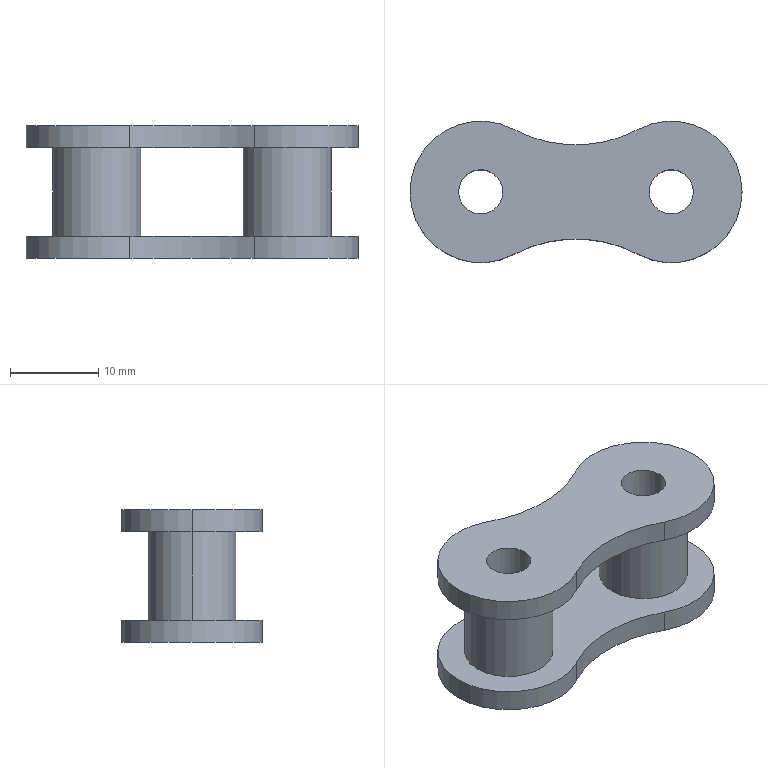Part | SolidWorks | 1 solid | 22 faces | box 37.56 x 16 x 15 mm | volume 3392 mm3 | cylinder 18 | plane 4 | commonest cylinder face diameters 16 x6 5 x4 10 x4 30 x4
STEP:
#1=CARTESIAN_POINT('',(3.75,-7.067,7.5));
#2=VERTEX_POINT('',#1);
#3=CARTESIAN_POINT('',(-8.,0.,7.5));
#4=VERTEX_POINT('',#3);
#5=CARTESIAN_POINT('',(0.,0.,7.5));
#6=DIRECTION('',(0.,0.,-1.));
#7=DIRECTION('',(-1.,0.,0.));
#8=AXIS2_PLACEMENT_3D('',#5,#6,#7);
#9=CIRCLE('',#8,8.);
#10=EDGE_CURVE('',#2,#4,#9,.T.);
#11=ORIENTED_EDGE('',*,*,#10,.T.);
#12=CARTESIAN_POINT('',(-8.,0.,5.));
#13=VERTEX_POINT('',#12);
#14=CARTESIAN_POINT('',(-8.,0.,7.5));
#15=DIRECTION('',(0.,0.,-1.));
#16=VECTOR('',#15,1000.);
#17=LINE('',#14,#16);
#18=EDGE_CURVE('',#4,#13,#17,.T.);
#19=ORIENTED_EDGE('',*,*,#18,.T.);
#20=CARTESIAN_POINT('',(3.75,-7.067,5.));
#21=VERTEX_POINT('',#20);
#22=CARTESIAN_POINT('',(0.,0.,5.));
#23=DIRECTION('',(0.,0.,-1.));
#24=DIRECTION('',(-1.,0.,0.));
#25=AXIS2_PLACEMENT_3D('',#22,#23,#24);
#26=CIRCLE('',#25,8.);
#27=EDGE_CURVE('',#21,#13,#26,.T.);
#28=ORIENTED_EDGE('',*,*,#27,.F.);
#29=CARTESIAN_POINT('',(3.75,-7.067,7.5));
#30=DIRECTION('',(0.,0.,-1.));
#31=VECTOR('',#30,1000.);
#32=LINE('',#29,#31);
#33=EDGE_CURVE('',#2,#21,#32,.T.);
#34=ORIENTED_EDGE('',*,*,#33,.F.);
#35=EDGE_LOOP('',(#11,#19,#28,#34));
#36=FACE_OUTER_BOUND('',#35,.T.);
#37=CARTESIAN_POINT('',(0.,0.,7.5));
#38=DIRECTION('',(0.,0.,-1.));
#39=DIRECTION('',(-1.,0.,0.));
#40=AXIS2_PLACEMENT_3D('',#37,#38,#39);
#41=CYLINDRICAL_SURFACE('',#40,8.);
#42=ADVANCED_FACE('',(#36),#41,.T.);
#43=CARTESIAN_POINT('',(26.56,0.,5.));
#44=VERTEX_POINT('',#43);
#45=CARTESIAN_POINT('',(16.56,0.,5.));
#46=VERTEX_POINT('',#45);
#47=CARTESIAN_POINT('',(21.56,0.,5.));
#48=DIRECTION('',(0.,0.,1.));
#49=DIRECTION('',(1.,0.,0.));
#50=AXIS2_PLACEMENT_3D('',#47,#48,#49);
#51=CIRCLE('',#50,5.);
#52=EDGE_CURVE('',#44,#46,#51,.T.);
#53=ORIENTED_EDGE('',*,*,#52,.F.);
#54=CARTESIAN_POINT('',(26.56,0.,-5.));
#55=VERTEX_POINT('',#54);
#56=CARTESIAN_POINT('',(26.56,0.,5.));
#57=DIRECTION('',(0.,0.,-1.));
#58=VECTOR('',#57,1000.);
#59=LINE('',#56,#58);
#60=EDGE_CURVE('',#44,#55,#59,.T.);
#61=ORIENTED_EDGE('',*,*,#60,.T.);
#62=CARTESIAN_POINT('',(16.56,0.,-5.));
#63=VERTEX_POINT('',#62);
#64=CARTESIAN_POINT('',(21.56,0.,-5.));
#65=DIRECTION('',(0.,0.,1.));
#66=DIRECTION('',(-1.,0.,0.));
#67=AXIS2_PLACEMENT_3D('',#64,#65,#66);
#68=CIRCLE('',#67,5.);
#69=EDGE_CURVE('',#55,#63,#68,.T.);
#70=ORIENTED_EDGE('',*,*,#69,.T.);
#71=CARTESIAN_POINT('',(16.56,0.,5.));
#72=DIRECTION('',(0.,0.,-1.));
#73=VECTOR('',#72,1000.);
#74=LINE('',#71,#73);
#75=EDGE_CURVE('',#46,#63,#74,.T.);
#76=ORIENTED_EDGE('',*,*,#75,.F.);
#77=EDGE_LOOP('',(#53,#61,#70,#76));
#78=FACE_OUTER_BOUND('',#77,.T.);
#79=CARTESIAN_POINT('',(21.56,0.,5.));
#80=DIRECTION('',(0.,0.,-1.));
#81=DIRECTION('',(-1.,0.,0.));
#82=AXIS2_PLACEMENT_3D('',#79,#80,#81);
#83=CYLINDRICAL_SURFACE('',#82,5.);
#84=ADVANCED_FACE('',(#78),#83,.T.);
#85=CARTESIAN_POINT('',(24.06,0.,-7.5));
#86=VERTEX_POINT('',#85);
#87=CARTESIAN_POINT('',(19.06,0.,-7.5));
#88=VERTEX_POINT('',#87);
#89=CARTESIAN_POINT('',(21.56,0.,-7.5));
#90=DIRECTION('',(0.,0.,-1.));
#91=DIRECTION('',(-1.,0.,0.));
#92=AXIS2_PLACEMENT_3D('',#89,#90,#91);
#93=CIRCLE('',#92,2.5);
#94=EDGE_CURVE('',#86,#88,#93,.T.);
#95=ORIENTED_EDGE('',*,*,#94,.T.);
#96=CARTESIAN_POINT('',(19.06,0.,7.5));
#97=VERTEX_POINT('',#96);
#98=CARTESIAN_POINT('',(19.06,0.,-7.5));
#99=DIRECTION('',(0.,0.,1.));
#100=VECTOR('',#99,1000.);
#101=LINE('',#98,#100);
#102=EDGE_CURVE('',#88,#97,#101,.T.);
#103=ORIENTED_EDGE('',*,*,#102,.T.);
#104=CARTESIAN_POINT('',(24.06,0.,7.5));
#105=VERTEX_POINT('',#104);
#106=CARTESIAN_POINT('',(21.56,0.,7.5));
#107=DIRECTION('',(0.,0.,-1.));
#108=DIRECTION('',(-1.,0.,0.));
#109=AXIS2_PLACEMENT_3D('',#106,#107,#108);
#110=CIRCLE('',#109,2.5);
#111=EDGE_CURVE('',#105,#97,#110,.T.);
#112=ORIENTED_EDGE('',*,*,#111,.F.);
#113=CARTESIAN_POINT('',(24.06,0.,-7.5));
#114=DIRECTION('',(0.,0.,1.));
#115=VECTOR('',#114,1000.);
#116=LINE('',#113,#115);
#117=EDGE_CURVE('',#86,#105,#116,.T.);
#118=ORIENTED_EDGE('',*,*,#117,.F.);
#119=EDGE_LOOP('',(#95,#103,#112,#118));
#120=FACE_OUTER_BOUND('',#119,.T.);
#121=CARTESIAN_POINT('',(21.56,0.,-7.5));
#122=DIRECTION('',(0.,0.,1.));
#123=DIRECTION('',(1.,0.,0.));
#124=AXIS2_PLACEMENT_3D('',#121,#122,#123);
#125=CYLINDRICAL_SURFACE('',#124,2.5);
#126=ADVANCED_FACE('',(#120),#125,.F.);
#127=CARTESIAN_POINT('',(29.56,0.,-7.5));
#128=VERTEX_POINT('',#127);
#129=CARTESIAN_POINT('',(17.81,-7.067,-7.5));
#130=VERTEX_POINT('',#129);
#131=CARTESIAN_POINT('',(21.56,0.,-7.5));
#132=DIRECTION('',(0.,0.,-1.));
#133=DIRECTION('',(-1.,0.,0.));
#134=AXIS2_PLACEMENT_3D('',#131,#132,#133);
#135=CIRCLE('',#134,8.);
#136=EDGE_CURVE('',#128,#130,#135,.T.);
#137=ORIENTED_EDGE('',*,*,#136,.F.);
#138=CARTESIAN_POINT('',(29.56,0.,-5.));
#139=VERTEX_POINT('',#138);
#140=CARTESIAN_POINT('',(29.56,0.,-7.5));
#141=DIRECTION('',(0.,0.,1.));
#142=VECTOR('',#141,1000.);
#143=LINE('',#140,#142);
#144=EDGE_CURVE('',#128,#139,#143,.T.);
#145=ORIENTED_EDGE('',*,*,#144,.T.);
#146=CARTESIAN_POINT('',(17.81,-7.067,-5.));
#147=VERTEX_POINT('',#146);
#148=CARTESIAN_POINT('',(21.56,0.,-5.));
#149=DIRECTION('',(0.,0.,-1.));
#150=DIRECTION('',(-1.,0.,0.));
#151=AXIS2_PLACEMENT_3D('',#148,#149,#150);
#152=CIRCLE('',#151,8.);
#153=EDGE_CURVE('',#139,#147,#152,.T.);
#154=ORIENTED_EDGE('',*,*,#153,.T.);
#155=CARTESIAN_POINT('',(17.81,-7.067,-7.5));
#156=DIRECTION('',(0.,0.,1.));
#157=VECTOR('',#156,1000.);
#158=LINE('',#155,#157);
#159=EDGE_CURVE('',#130,#147,#158,.T.);
#160=ORIENTED_EDGE('',*,*,#159,.F.);
#161=EDGE_LOOP('',(#137,#145,#154,#160));
#162=FACE_OUTER_BOUND('',#161,.T.);
#163=CARTESIAN_POINT('',(21.56,0.,-7.5));
#164=DIRECTION('',(0.,0.,1.));
#165=DIRECTION('',(1.,0.,0.));
#166=AXIS2_PLACEMENT_3D('',#163,#164,#165);
#167=CYLINDRICAL_SURFACE('',#166,8.);
#168=ADVANCED_FACE('',(#162),#167,.T.);
#169=CARTESIAN_POINT('',(2.5,0.,7.5));
#170=VERTEX_POINT('',#169);
#171=CARTESIAN_POINT('',(-2.5,0.,7.5));
#172=VERTEX_POINT('',#171);
#173=CARTESIAN_POINT('',(0.,0.,7.5));
#174=DIRECTION('',(0.,0.,-1.));
#175=DIRECTION('',(-1.,0.,0.));
#176=AXIS2_PLACEMENT_3D('',#173,#174,#175);
#177=CIRCLE('',#176,2.5);
#178=EDGE_CURVE('',#170,#172,#177,.T.);
#179=ORIENTED_EDGE('',*,*,#178,.F.);
#180=CARTESIAN_POINT('',(2.5,0.,-7.5));
#181=VERTEX_POINT('',#180);
#182=CARTESIAN_POINT('',(2.5,0.,5.));
#183=DIRECTION('',(0.,0.,-1.));
#184=VECTOR('',#183,1000.);
#185=LINE('',#182,#184);
#186=EDGE_CURVE('',#170,#181,#185,.T.);
#187=ORIENTED_EDGE('',*,*,#186,.T.);
#188=CARTESIAN_POINT('',(-2.5,0.,-7.5));
#189=VERTEX_POINT('',#188);
#190=CARTESIAN_POINT('',(0.,0.,-7.5));
#191=DIRECTION('',(0.,0.,-1.));
#192=DIRECTION('',(-1.,0.,0.));
#193=AXIS2_PLACEMENT_3D('',#190,#191,#192);
#194=CIRCLE('',#193,2.5);
#195=EDGE_CURVE('',#181,#189,#194,.T.);
#196=ORIENTED_EDGE('',*,*,#195,.T.);
#197=CARTESIAN_POINT('',(-2.5,0.,5.));
#198=DIRECTION('',(0.,0.,-1.));
#199=VECTOR('',#198,1000.);
#200=LINE('',#197,#199);
#201=EDGE_CURVE('',#172,#189,#200,.T.);
#202=ORIENTED_EDGE('',*,*,#201,.F.);
#203=EDGE_LOOP('',(#179,#187,#196,#202));
#204=FACE_OUTER_BOUND('',#203,.T.);
#205=CARTESIAN_POINT('',(0.,0.,5.));
#206=DIRECTION('',(0.,0.,-1.));
#207=DIRECTION('',(-1.,0.,0.));
#208=AXIS2_PLACEMENT_3D('',#205,#206,#207);
#209=CYLINDRICAL_SURFACE('',#208,2.5);
#210=ADVANCED_FACE('',(#204),#209,.F.);
#211=CARTESIAN_POINT('',(5.,0.,5.));
#212=VERTEX_POINT('',#211);
#213=CARTESIAN_POINT('',(-5.,0.,5.));
#214=VERTEX_POINT('',#213);
#215=CARTESIAN_POINT('',(0.,0.,5.));
#216=DIRECTION('',(0.,0.,1.));
#217=DIRECTION('',(1.,0.,0.));
#218=AXIS2_PLACEMENT_3D('',#215,#216,#217);
#219=CIRCLE('',#218,5.);
#220=EDGE_CURVE('',#212,#214,#219,.T.);
#221=ORIENTED_EDGE('',*,*,#220,.F.);
#222=CARTESIAN_POINT('',(5.,0.,-5.));
#223=VERTEX_POINT('',#222);
#224=CARTESIAN_POINT('',(5.,0.,5.));
#225=DIRECTION('',(0.,0.,-1.));
#226=VECTOR('',#225,1000.);
#227=LINE('',#224,#226);
#228=EDGE_CURVE('',#212,#223,#227,.T.);
#229=ORIENTED_EDGE('',*,*,#228,.T.);
#230=CARTESIAN_POINT('',(-5.,0.,-5.));
#231=VERTEX_POINT('',#230);
#232=CARTESIAN_POINT('',(0.,0.,-5.));
#233=DIRECTION('',(0.,0.,1.));
#234=DIRECTION('',(1.,0.,0.));
#235=AXIS2_PLACEMENT_3D('',#232,#233,#234);
#236=CIRCLE('',#235,5.);
#237=EDGE_CURVE('',#223,#231,#236,.T.);
#238=ORIENTED_EDGE('',*,*,#237,.T.);
#239=CARTESIAN_POINT('',(-5.,0.,5.));
#240=DIRECTION('',(0.,0.,-1.));
#241=VECTOR('',#240,1000.);
#242=LINE('',#239,#241);
#243=EDGE_CURVE('',#214,#231,#242,.T.);
#244=ORIENTED_EDGE('',*,*,#243,.F.);
#245=EDGE_LOOP('',(#221,#229,#238,#244));
#246=FACE_OUTER_BOUND('',#245,.T.);
#247=CARTESIAN_POINT('',(0.,0.,5.));
#248=DIRECTION('',(0.,0.,-1.));
#249=DIRECTION('',(-1.,0.,0.));
#250=AXIS2_PLACEMENT_3D('',#247,#248,#249);
#251=CYLINDRICAL_SURFACE('',#250,5.);
#252=ADVANCED_FACE('',(#246),#251,.T.);
#253=CARTESIAN_POINT('',(3.75,7.067,-5.));
#254=VERTEX_POINT('',#253);
#255=CARTESIAN_POINT('',(17.81,7.067,-5.));
#256=VERTEX_POINT('',#255);
#257=CARTESIAN_POINT('',(10.78,20.317,-5.));
#258=DIRECTION('',(0.,0.,1.));
#259=DIRECTION('',(-1.,0.,0.));
#260=AXIS2_PLACEMENT_3D('',#257,#258,#259);
#261=CIRCLE('',#260,15.);
#262=EDGE_CURVE('',#254,#256,#261,.T.);
#263=ORIENTED_EDGE('',*,*,#262,.F.);
#264=CARTESIAN_POINT('',(3.75,-7.067,-5.));
#265=VERTEX_POINT('',#264);
#266=CARTESIAN_POINT('',(0.,0.,-5.));
#267=DIRECTION('',(0.,0.,-1.));
#268=DIRECTION('',(-1.,0.,0.));
#269=AXIS2_PLACEMENT_3D('',#266,#267,#268);
#270=CIRCLE('',#269,8.);
#271=EDGE_CURVE('',#265,#254,#270,.T.);
#272=ORIENTED_EDGE('',*,*,#271,.F.);
#273=CARTESIAN_POINT('',(10.78,-20.317,-5.));
#274=DIRECTION('',(0.,0.,1.));
#275=DIRECTION('',(1.,0.,0.));
#276=AXIS2_PLACEMENT_3D('',#273,#274,#275);
#277=CIRCLE('',#276,15.);
#278=EDGE_CURVE('',#147,#265,#277,.T.);
#279=ORIENTED_EDGE('',*,*,#278,.F.);
#280=ORIENTED_EDGE('',*,*,#153,.F.);
#281=CARTESIAN_POINT('',(21.56,0.,-5.));
#282=DIRECTION('',(0.,0.,-1.));
#283=DIRECTION('',(-1.,0.,0.));
#284=AXIS2_PLACEMENT_3D('',#281,#282,#283);
#285=CIRCLE('',#284,8.);
#286=EDGE_CURVE('',#256,#139,#285,.T.);
#287=ORIENTED_EDGE('',*,*,#286,.F.);
#288=EDGE_LOOP('',(#263,#272,#279,#280,#287));
#289=FACE_OUTER_BOUND('',#288,.T.);
#290=CARTESIAN_POINT('',(0.,0.,-5.));
#291=DIRECTION('',(0.,0.,1.));
#292=DIRECTION('',(1.,0.,0.));
#293=AXIS2_PLACEMENT_3D('',#290,#291,#292);
#294=CIRCLE('',#293,5.);
#295=EDGE_CURVE('',#231,#223,#294,.T.);
#296=ORIENTED_EDGE('',*,*,#295,.F.);
#297=ORIENTED_EDGE('',*,*,#237,.F.);
#298=EDGE_LOOP('',(#296,#297));
#299=FACE_BOUND('',#298,.T.);
#300=CARTESIAN_POINT('',(21.56,0.,-5.));
#301=DIRECTION('',(0.,0.,1.));
#302=DIRECTION('',(-1.,0.,0.));
#303=AXIS2_PLACEMENT_3D('',#300,#301,#302);
#304=CIRCLE('',#303,5.);
#305=EDGE_CURVE('',#63,#55,#304,.T.);
#306=ORIENTED_EDGE('',*,*,#305,.F.);
#307=ORIENTED_EDGE('',*,*,#69,.F.);
#308=EDGE_LOOP('',(#306,#307));
#309=FACE_BOUND('',#308,.T.);
#310=CARTESIAN_POINT('',(5.39,10.159,-5.));
#311=DIRECTION('',(0.,0.,-1.));
#312=DIRECTION('',(-1.,0.,0.));
#313=AXIS2_PLACEMENT_3D('',#310,#311,#312);
#314=PLANE('',#313);
#315=ADVANCED_FACE('',(#289,#299,#309),#314,.F.);
#316=ORIENTED_EDGE('',*,*,#228,.F.);
#317=CARTESIAN_POINT('',(0.,0.,5.));
#318=DIRECTION('',(0.,0.,1.));
#319=DIRECTION('',(1.,0.,0.));
#320=AXIS2_PLACEMENT_3D('',#317,#318,#319);
#321=CIRCLE('',#320,5.);
#322=EDGE_CURVE('',#214,#212,#321,.T.);
#323=ORIENTED_EDGE('',*,*,#322,.F.);
#324=ORIENTED_EDGE('',*,*,#243,.T.);
#325=ORIENTED_EDGE('',*,*,#295,.T.);
#326=EDGE_LOOP('',(#316,#323,#324,#325));
#327=FACE_OUTER_BOUND('',#326,.T.);
#328=CARTESIAN_POINT('',(0.,0.,5.));
#329=DIRECTION('',(0.,0.,-1.));
#330=DIRECTION('',(-1.,0.,0.));
#331=AXIS2_PLACEMENT_3D('',#328,#329,#330);
#332=CYLINDRICAL_SURFACE('',#331,5.);
#333=ADVANCED_FACE('',(#327),#332,.T.);
#334=ORIENTED_EDGE('',*,*,#186,.F.);
#335=CARTESIAN_POINT('',(0.,0.,7.5));
#336=DIRECTION('',(0.,0.,-1.));
#337=DIRECTION('',(-1.,0.,0.));
#338=AXIS2_PLACEMENT_3D('',#335,#336,#337);
#339=CIRCLE('',#338,2.5);
#340=EDGE_CURVE('',#172,#170,#339,.T.);
#341=ORIENTED_EDGE('',*,*,#340,.F.);
#342=ORIENTED_EDGE('',*,*,#201,.T.);
#343=CARTESIAN_POINT('',(0.,0.,-7.5));
#344=DIRECTION('',(0.,0.,-1.));
#345=DIRECTION('',(-1.,0.,0.));
#346=AXIS2_PLACEMENT_3D('',#343,#344,#345);
#347=CIRCLE('',#346,2.5);
#348=EDGE_CURVE('',#189,#181,#347,.T.);
#349=ORIENTED_EDGE('',*,*,#348,.T.);
#350=EDGE_LOOP('',(#334,#341,#342,#349));
#351=FACE_OUTER_BOUND('',#350,.T.);
#352=CARTESIAN_POINT('',(0.,0.,5.));
#353=DIRECTION('',(0.,0.,-1.));
#354=DIRECTION('',(-1.,0.,0.));
#355=AXIS2_PLACEMENT_3D('',#352,#353,#354);
#356=CYLINDRICAL_SURFACE('',#355,2.5);
#357=ADVANCED_FACE('',(#351),#356,.F.);
#358=ORIENTED_EDGE('',*,*,#94,.F.);
#359=CARTESIAN_POINT('',(21.56,0.,-7.5));
#360=DIRECTION('',(0.,0.,-1.));
#361=DIRECTION('',(-1.,0.,0.));
#362=AXIS2_PLACEMENT_3D('',#359,#360,#361);
#363=CIRCLE('',#362,2.5);
#364=EDGE_CURVE('',#88,#86,#363,.T.);
#365=ORIENTED_EDGE('',*,*,#364,.F.);
#366=EDGE_LOOP('',(#358,#365));
#367=FACE_BOUND('',#366,.T.);
#368=CARTESIAN_POINT('',(3.75,7.067,-7.5));
#369=VERTEX_POINT('',#368);
#370=CARTESIAN_POINT('',(17.81,7.067,-7.5));
#371=VERTEX_POINT('',#370);
#372=CARTESIAN_POINT('',(10.78,20.317,-7.5));
#373=DIRECTION('',(0.,0.,1.));
#374=DIRECTION('',(-1.,0.,0.));
#375=AXIS2_PLACEMENT_3D('',#372,#373,#374);
#376=CIRCLE('',#375,15.);
#377=EDGE_CURVE('',#369,#371,#376,.T.);
#378=ORIENTED_EDGE('',*,*,#377,.T.);
#379=CARTESIAN_POINT('',(21.56,0.,-7.5));
#380=DIRECTION('',(0.,0.,-1.));
#381=DIRECTION('',(-1.,0.,0.));
#382=AXIS2_PLACEMENT_3D('',#379,#380,#381);
#383=CIRCLE('',#382,8.);
#384=EDGE_CURVE('',#371,#128,#383,.T.);
#385=ORIENTED_EDGE('',*,*,#384,.T.);
#386=ORIENTED_EDGE('',*,*,#136,.T.);
#387=CARTESIAN_POINT('',(3.75,-7.067,-7.5));
#388=VERTEX_POINT('',#387);
#389=CARTESIAN_POINT('',(10.78,-20.317,-7.5));
#390=DIRECTION('',(0.,0.,1.));
#391=DIRECTION('',(1.,0.,0.));
#392=AXIS2_PLACEMENT_3D('',#389,#390,#391);
#393=CIRCLE('',#392,15.);
#394=EDGE_CURVE('',#130,#388,#393,.T.);
#395=ORIENTED_EDGE('',*,*,#394,.T.);
#396=CARTESIAN_POINT('',(0.,0.,-7.5));
#397=DIRECTION('',(0.,0.,-1.));
#398=DIRECTION('',(-1.,0.,0.));
#399=AXIS2_PLACEMENT_3D('',#396,#397,#398);
#400=CIRCLE('',#399,8.);
#401=EDGE_CURVE('',#388,#369,#400,.T.);
#402=ORIENTED_EDGE('',*,*,#401,.T.);
#403=EDGE_LOOP('',(#378,#385,#386,#395,#402));
#404=FACE_OUTER_BOUND('',#403,.T.);
#405=ORIENTED_EDGE('',*,*,#348,.F.);
#406=ORIENTED_EDGE('',*,*,#195,.F.);
#407=EDGE_LOOP('',(#405,#406));
#408=FACE_BOUND('',#407,.T.);
#409=CARTESIAN_POINT('',(5.39,10.159,-7.5));
#410=DIRECTION('',(0.,0.,-1.));
#411=DIRECTION('',(-1.,0.,0.));
#412=AXIS2_PLACEMENT_3D('',#409,#410,#411);
#413=PLANE('',#412);
#414=ADVANCED_FACE('',(#367,#404,#408),#413,.T.);
#415=ORIENTED_EDGE('',*,*,#262,.T.);
#416=CARTESIAN_POINT('',(17.81,7.067,-7.5));
#417=DIRECTION('',(0.,0.,1.));
#418=VECTOR('',#417,1000.);
#419=LINE('',#416,#418);
#420=EDGE_CURVE('',#371,#256,#419,.T.);
#421=ORIENTED_EDGE('',*,*,#420,.F.);
#422=ORIENTED_EDGE('',*,*,#377,.F.);
#423=CARTESIAN_POINT('',(3.75,7.067,-7.5));
#424=DIRECTION('',(0.,0.,1.));
#425=VECTOR('',#424,1000.);
#426=LINE('',#423,#425);
#427=EDGE_CURVE('',#369,#254,#426,.T.);
#428=ORIENTED_EDGE('',*,*,#427,.T.);
#429=EDGE_LOOP('',(#415,#421,#422,#428));
#430=FACE_OUTER_BOUND('',#429,.T.);
#431=CARTESIAN_POINT('',(10.78,20.317,-7.5));
#432=DIRECTION('',(0.,0.,1.));
#433=DIRECTION('',(1.,0.,0.));
#434=AXIS2_PLACEMENT_3D('',#431,#432,#433);
#435=CYLINDRICAL_SURFACE('',#434,15.);
#436=ADVANCED_FACE('',(#430),#435,.F.);
#437=ORIENTED_EDGE('',*,*,#144,.F.);
#438=ORIENTED_EDGE('',*,*,#384,.F.);
#439=ORIENTED_EDGE('',*,*,#420,.T.);
#440=ORIENTED_EDGE('',*,*,#286,.T.);
#441=EDGE_LOOP('',(#437,#438,#439,#440));
#442=FACE_OUTER_BOUND('',#441,.T.);
#443=CARTESIAN_POINT('',(21.56,0.,-7.5));
#444=DIRECTION('',(0.,0.,1.));
#445=DIRECTION('',(1.,0.,0.));
#446=AXIS2_PLACEMENT_3D('',#443,#444,#445);
#447=CYLINDRICAL_SURFACE('',#446,8.);
#448=ADVANCED_FACE('',(#442),#447,.T.);
#449=ORIENTED_EDGE('',*,*,#278,.T.);
#450=CARTESIAN_POINT('',(3.75,-7.067,-7.5));
#451=DIRECTION('',(0.,0.,1.));
#452=VECTOR('',#451,1000.);
#453=LINE('',#450,#452);
#454=EDGE_CURVE('',#388,#265,#453,.T.);
#455=ORIENTED_EDGE('',*,*,#454,.F.);
#456=ORIENTED_EDGE('',*,*,#394,.F.);
#457=ORIENTED_EDGE('',*,*,#159,.T.);
#458=EDGE_LOOP('',(#449,#455,#456,#457));
#459=FACE_OUTER_BOUND('',#458,.T.);
#460=CARTESIAN_POINT('',(10.78,-20.317,-7.5));
#461=DIRECTION('',(0.,0.,1.));
#462=DIRECTION('',(1.,0.,0.));
#463=AXIS2_PLACEMENT_3D('',#460,#461,#462);
#464=CYLINDRICAL_SURFACE('',#463,15.);
#465=ADVANCED_FACE('',(#459),#464,.F.);
#466=ORIENTED_EDGE('',*,*,#271,.T.);
#467=ORIENTED_EDGE('',*,*,#427,.F.);
#468=ORIENTED_EDGE('',*,*,#401,.F.);
#469=ORIENTED_EDGE('',*,*,#454,.T.);
#470=EDGE_LOOP('',(#466,#467,#468,#469));
#471=FACE_OUTER_BOUND('',#470,.T.);
#472=CARTESIAN_POINT('',(0.,0.,-7.5));
#473=DIRECTION('',(0.,0.,1.));
#474=DIRECTION('',(1.,0.,0.));
#475=AXIS2_PLACEMENT_3D('',#472,#473,#474);
#476=CYLINDRICAL_SURFACE('',#475,8.);
#477=ADVANCED_FACE('',(#471),#476,.T.);
#478=ORIENTED_EDGE('',*,*,#102,.F.);
#479=ORIENTED_EDGE('',*,*,#364,.T.);
#480=ORIENTED_EDGE('',*,*,#117,.T.);
#481=CARTESIAN_POINT('',(21.56,0.,7.5));
#482=DIRECTION('',(0.,0.,-1.));
#483=DIRECTION('',(-1.,0.,0.));
#484=AXIS2_PLACEMENT_3D('',#481,#482,#483);
#485=CIRCLE('',#484,2.5);
#486=EDGE_CURVE('',#97,#105,#485,.T.);
#487=ORIENTED_EDGE('',*,*,#486,.F.);
#488=EDGE_LOOP('',(#478,#479,#480,#487));
#489=FACE_OUTER_BOUND('',#488,.T.);
#490=CARTESIAN_POINT('',(21.56,0.,-7.5));
#491=DIRECTION('',(0.,0.,1.));
#492=DIRECTION('',(1.,0.,0.));
#493=AXIS2_PLACEMENT_3D('',#490,#491,#492);
#494=CYLINDRICAL_SURFACE('',#493,2.5);
#495=ADVANCED_FACE('',(#489),#494,.F.);
#496=ORIENTED_EDGE('',*,*,#60,.F.);
#497=CARTESIAN_POINT('',(21.56,0.,5.));
#498=DIRECTION('',(0.,0.,1.));
#499=DIRECTION('',(1.,0.,0.));
#500=AXIS2_PLACEMENT_3D('',#497,#498,#499);
#501=CIRCLE('',#500,5.);
#502=EDGE_CURVE('',#46,#44,#501,.T.);
#503=ORIENTED_EDGE('',*,*,#502,.F.);
#504=ORIENTED_EDGE('',*,*,#75,.T.);
#505=ORIENTED_EDGE('',*,*,#305,.T.);
#506=EDGE_LOOP('',(#496,#503,#504,#505));
#507=FACE_OUTER_BOUND('',#506,.T.);
#508=CARTESIAN_POINT('',(21.56,0.,5.));
#509=DIRECTION('',(0.,0.,-1.));
#510=DIRECTION('',(-1.,0.,0.));
#511=AXIS2_PLACEMENT_3D('',#508,#509,#510);
#512=CYLINDRICAL_SURFACE('',#511,5.);
#513=ADVANCED_FACE('',(#507),#512,.T.);
#514=CARTESIAN_POINT('',(3.75,7.067,5.));
#515=VERTEX_POINT('',#514);
#516=CARTESIAN_POINT('',(17.81,7.067,5.));
#517=VERTEX_POINT('',#516);
#518=CARTESIAN_POINT('',(10.78,20.317,5.));
#519=DIRECTION('',(0.,0.,1.));
#520=DIRECTION('',(-1.,0.,0.));
#521=AXIS2_PLACEMENT_3D('',#518,#519,#520);
#522=CIRCLE('',#521,15.);
#523=EDGE_CURVE('',#515,#517,#522,.T.);
#524=ORIENTED_EDGE('',*,*,#523,.F.);
#525=CARTESIAN_POINT('',(3.75,7.067,7.5));
#526=VERTEX_POINT('',#525);
#527=CARTESIAN_POINT('',(3.75,7.067,7.5));
#528=DIRECTION('',(0.,0.,-1.));
#529=VECTOR('',#528,1000.);
#530=LINE('',#527,#529);
#531=EDGE_CURVE('',#526,#515,#530,.T.);
#532=ORIENTED_EDGE('',*,*,#531,.F.);
#533=CARTESIAN_POINT('',(17.81,7.067,7.5));
#534=VERTEX_POINT('',#533);
#535=CARTESIAN_POINT('',(10.78,20.317,7.5));
#536=DIRECTION('',(0.,0.,1.));
#537=DIRECTION('',(-1.,0.,0.));
#538=AXIS2_PLACEMENT_3D('',#535,#536,#537);
#539=CIRCLE('',#538,15.);
#540=EDGE_CURVE('',#526,#534,#539,.T.);
#541=ORIENTED_EDGE('',*,*,#540,.T.);
#542=CARTESIAN_POINT('',(17.81,7.067,7.5));
#543=DIRECTION('',(0.,0.,-1.));
#544=VECTOR('',#543,1000.);
#545=LINE('',#542,#544);
#546=EDGE_CURVE('',#534,#517,#545,.T.);
#547=ORIENTED_EDGE('',*,*,#546,.T.);
#548=EDGE_LOOP('',(#524,#532,#541,#547));
#549=FACE_OUTER_BOUND('',#548,.T.);
#550=CARTESIAN_POINT('',(10.78,20.317,7.5));
#551=DIRECTION('',(0.,0.,-1.));
#552=DIRECTION('',(-1.,0.,0.));
#553=AXIS2_PLACEMENT_3D('',#550,#551,#552);
#554=CYLINDRICAL_SURFACE('',#553,15.);
#555=ADVANCED_FACE('',(#549),#554,.F.);
#556=ORIENTED_EDGE('',*,*,#18,.F.);
#557=CARTESIAN_POINT('',(0.,0.,7.5));
#558=DIRECTION('',(0.,0.,-1.));
#559=DIRECTION('',(-1.,0.,0.));
#560=AXIS2_PLACEMENT_3D('',#557,#558,#559);
#561=CIRCLE('',#560,8.);
#562=EDGE_CURVE('',#4,#526,#561,.T.);
#563=ORIENTED_EDGE('',*,*,#562,.T.);
#564=ORIENTED_EDGE('',*,*,#531,.T.);
#565=CARTESIAN_POINT('',(0.,0.,5.));
#566=DIRECTION('',(0.,0.,-1.));
#567=DIRECTION('',(-1.,0.,0.));
#568=AXIS2_PLACEMENT_3D('',#565,#566,#567);
#569=CIRCLE('',#568,8.);
#570=EDGE_CURVE('',#13,#515,#569,.T.);
#571=ORIENTED_EDGE('',*,*,#570,.F.);
#572=EDGE_LOOP('',(#556,#563,#564,#571));
#573=FACE_OUTER_BOUND('',#572,.T.);
#574=CARTESIAN_POINT('',(0.,0.,7.5));
#575=DIRECTION('',(0.,0.,-1.));
#576=DIRECTION('',(-1.,0.,0.));
#577=AXIS2_PLACEMENT_3D('',#574,#575,#576);
#578=CYLINDRICAL_SURFACE('',#577,8.);
#579=ADVANCED_FACE('',(#573),#578,.T.);
#580=CARTESIAN_POINT('',(17.81,-7.067,5.));
#581=VERTEX_POINT('',#580);
#582=CARTESIAN_POINT('',(10.78,-20.317,5.));
#583=DIRECTION('',(0.,0.,1.));
#584=DIRECTION('',(1.,0.,0.));
#585=AXIS2_PLACEMENT_3D('',#582,#583,#584);
#586=CIRCLE('',#585,15.);
#587=EDGE_CURVE('',#581,#21,#586,.T.);
#588=ORIENTED_EDGE('',*,*,#587,.F.);
#589=CARTESIAN_POINT('',(17.81,-7.067,7.5));
#590=VERTEX_POINT('',#589);
#591=CARTESIAN_POINT('',(17.81,-7.067,7.5));
#592=DIRECTION('',(0.,0.,-1.));
#593=VECTOR('',#592,1000.);
#594=LINE('',#591,#593);
#595=EDGE_CURVE('',#590,#581,#594,.T.);
#596=ORIENTED_EDGE('',*,*,#595,.F.);
#597=CARTESIAN_POINT('',(10.78,-20.317,7.5));
#598=DIRECTION('',(0.,0.,1.));
#599=DIRECTION('',(1.,0.,0.));
#600=AXIS2_PLACEMENT_3D('',#597,#598,#599);
#601=CIRCLE('',#600,15.);
#602=EDGE_CURVE('',#590,#2,#601,.T.);
#603=ORIENTED_EDGE('',*,*,#602,.T.);
#604=ORIENTED_EDGE('',*,*,#33,.T.);
#605=EDGE_LOOP('',(#588,#596,#603,#604));
#606=FACE_OUTER_BOUND('',#605,.T.);
#607=CARTESIAN_POINT('',(10.78,-20.317,7.5));
#608=DIRECTION('',(0.,0.,-1.));
#609=DIRECTION('',(-1.,0.,0.));
#610=AXIS2_PLACEMENT_3D('',#607,#608,#609);
#611=CYLINDRICAL_SURFACE('',#610,15.);
#612=ADVANCED_FACE('',(#606),#611,.F.);
#613=CARTESIAN_POINT('',(21.56,0.,5.));
#614=DIRECTION('',(0.,0.,-1.));
#615=DIRECTION('',(-1.,0.,0.));
#616=AXIS2_PLACEMENT_3D('',#613,#614,#615);
#617=CIRCLE('',#616,8.);
#618=EDGE_CURVE('',#517,#581,#617,.T.);
#619=ORIENTED_EDGE('',*,*,#618,.F.);
#620=ORIENTED_EDGE('',*,*,#546,.F.);
#621=CARTESIAN_POINT('',(21.56,0.,7.5));
#622=DIRECTION('',(0.,0.,-1.));
#623=DIRECTION('',(-1.,0.,0.));
#624=AXIS2_PLACEMENT_3D('',#621,#622,#623);
#625=CIRCLE('',#624,8.);
#626=EDGE_CURVE('',#534,#590,#625,.T.);
#627=ORIENTED_EDGE('',*,*,#626,.T.);
#628=ORIENTED_EDGE('',*,*,#595,.T.);
#629=EDGE_LOOP('',(#619,#620,#627,#628));
#630=FACE_OUTER_BOUND('',#629,.T.);
#631=CARTESIAN_POINT('',(21.56,0.,7.5));
#632=DIRECTION('',(0.,0.,-1.));
#633=DIRECTION('',(-1.,0.,0.));
#634=AXIS2_PLACEMENT_3D('',#631,#632,#633);
#635=CYLINDRICAL_SURFACE('',#634,8.);
#636=ADVANCED_FACE('',(#630),#635,.T.);
#637=ORIENTED_EDGE('',*,*,#340,.T.);
#638=ORIENTED_EDGE('',*,*,#178,.T.);
#639=EDGE_LOOP('',(#637,#638));
#640=FACE_BOUND('',#639,.T.);
#641=ORIENTED_EDGE('',*,*,#111,.T.);
#642=ORIENTED_EDGE('',*,*,#486,.T.);
#643=EDGE_LOOP('',(#641,#642));
#644=FACE_BOUND('',#643,.T.);
#645=ORIENTED_EDGE('',*,*,#540,.F.);
#646=ORIENTED_EDGE('',*,*,#562,.F.);
#647=ORIENTED_EDGE('',*,*,#10,.F.);
#648=ORIENTED_EDGE('',*,*,#602,.F.);
#649=ORIENTED_EDGE('',*,*,#626,.F.);
#650=EDGE_LOOP('',(#645,#646,#647,#648,#649));
#651=FACE_OUTER_BOUND('',#650,.T.);
#652=CARTESIAN_POINT('',(5.39,10.159,7.5));
#653=DIRECTION('',(0.,0.,1.));
#654=DIRECTION('',(-1.,0.,0.));
#655=AXIS2_PLACEMENT_3D('',#652,#653,#654);
#656=PLANE('',#655);
#657=ADVANCED_FACE('',(#640,#644,#651),#656,.T.);
#658=ORIENTED_EDGE('',*,*,#322,.T.);
#659=ORIENTED_EDGE('',*,*,#220,.T.);
#660=EDGE_LOOP('',(#658,#659));
#661=FACE_BOUND('',#660,.T.);
#662=ORIENTED_EDGE('',*,*,#502,.T.);
#663=ORIENTED_EDGE('',*,*,#52,.T.);
#664=EDGE_LOOP('',(#662,#663));
#665=FACE_BOUND('',#664,.T.);
#666=ORIENTED_EDGE('',*,*,#523,.T.);
#667=ORIENTED_EDGE('',*,*,#618,.T.);
#668=ORIENTED_EDGE('',*,*,#587,.T.);
#669=ORIENTED_EDGE('',*,*,#27,.T.);
#670=ORIENTED_EDGE('',*,*,#570,.T.);
#671=EDGE_LOOP('',(#666,#667,#668,#669,#670));
#672=FACE_OUTER_BOUND('',#671,.T.);
#673=CARTESIAN_POINT('',(5.39,10.159,5.));
#674=DIRECTION('',(0.,0.,1.));
#675=DIRECTION('',(-1.,0.,0.));
#676=AXIS2_PLACEMENT_3D('',#673,#674,#675);
#677=PLANE('',#676);
#678=ADVANCED_FACE('',(#661,#665,#672),#677,.F.);
#679=CLOSED_SHELL('',(#42,#84,#126,#168,#210,#252,#315,#333,#357,#414,#436,#448,#465,#477,#495,#513,#555,#579,#612,#636,#657,#678));
#680=MANIFOLD_SOLID_BREP('',#679);
#681=CARTESIAN_POINT('',(0.,0.,0.));
#682=DIRECTION('',(0.,0.,1.));
#683=DIRECTION('',(1.,0.,0.));
#684=AXIS2_PLACEMENT_3D('',#681,#682,#683);
#685=(LENGTH_UNIT()NAMED_UNIT(*)SI_UNIT(.MILLI.,.METRE.));
#686=UNCERTAINTY_MEASURE_WITH_UNIT(LENGTH_MEASURE(0.00001),#685,'','');
#687=(NAMED_UNIT(*)PLANE_ANGLE_UNIT()SI_UNIT($,.RADIAN.));
#688=(NAMED_UNIT(*)SI_UNIT($,.STERADIAN.)SOLID_ANGLE_UNIT());
#689=(GEOMETRIC_REPRESENTATION_CONTEXT(3)GLOBAL_UNCERTAINTY_ASSIGNED_CONTEXT((#686))GLOBAL_UNIT_ASSIGNED_CONTEXT((#685,#687,#688))REPRESENTATION_CONTEXT('',''));
#690=ADVANCED_BREP_SHAPE_REPRESENTATION('',(#680,#684),#689);